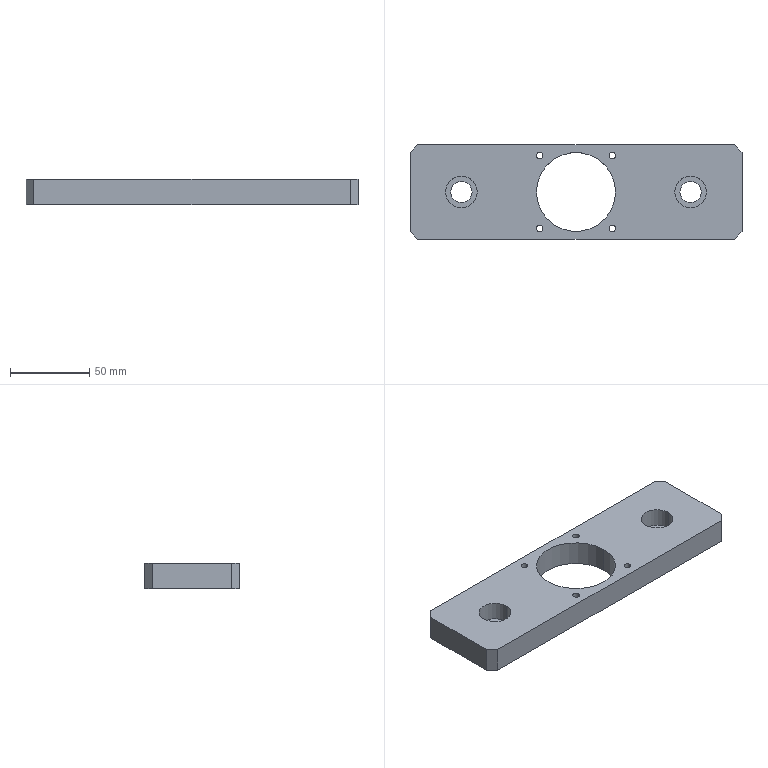Part | STEP file | fBY02F02M-00-24A | 1 solid | 30 faces | box 210 x 60 x 16 mm | volume 159812 mm3 | cylinder 18 | plane 12 | commonest cylinder face diameters 4.2 x8 13.5 x4 20 x4 50 x2